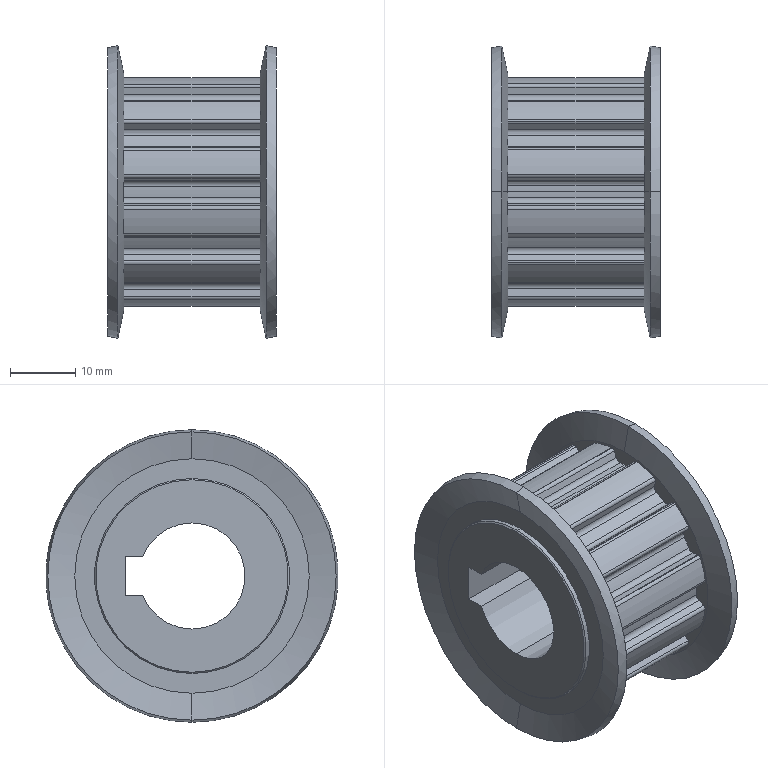Part | STEP file | ATPA12L075_A_N16_ATPA12L075-A-N14 | 1 solid | 147 faces | box 26 x 45 x 45 mm | volume 19221 mm3 | cylinder 99 | plane 34 | cone 14 | commonest cylinder face diameters 1.72 x32 1.06 x30 31.36 x14 35.62 x12 4.134 x4 30 x4